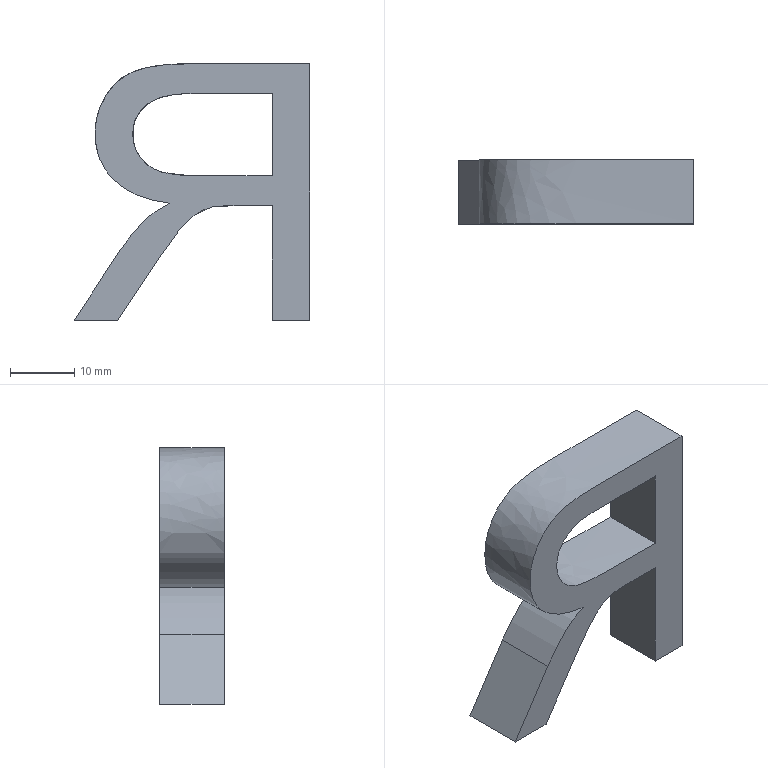Part | NX | features solid 2 | 1 solid | 13 faces | box 36.727 x 10 x 40 mm | volume 6487 mm3 | plane 8 | spline 5
STEP:
#1=CARTESIAN_POINT('',(182.141,850.,-144.665));
#2=VERTEX_POINT('',#1);
#3=CARTESIAN_POINT('',(182.141,850.,-157.484));
#4=VERTEX_POINT('',#3);
#5=CARTESIAN_POINT('',(182.141,850.,-144.665));
#6=CARTESIAN_POINT('',(182.141,850.,-148.938));
#7=CARTESIAN_POINT('',(182.141,850.,-153.211));
#8=CARTESIAN_POINT('',(182.141,850.,-157.484));
#9=B_SPLINE_CURVE_WITH_KNOTS('',3,(#5,#6,#7,#8),.UNSPECIFIED.,.F.,.F.,(4,4),(0.,0.1987),.PIECEWISE_BEZIER_KNOTS.);
#10=EDGE_CURVE('',#2,#4,#9,.T.);
#11=ORIENTED_EDGE('',*,*,#10,.F.);
#12=CARTESIAN_POINT('',(182.141,860.,-144.665));
#13=VERTEX_POINT('',#12);
#14=CARTESIAN_POINT('',(182.141,860.,-144.665));
#15=DIRECTION('',(0.,-1.,0.));
#16=VECTOR('',#15,1000.);
#17=LINE('',#14,#16);
#18=EDGE_CURVE('',#2,#13,#17,.F.);
#19=ORIENTED_EDGE('',*,*,#18,.T.);
#20=CARTESIAN_POINT('',(182.141,860.,-157.484));
#21=VERTEX_POINT('',#20);
#22=CARTESIAN_POINT('',(182.141,860.,-144.665));
#23=CARTESIAN_POINT('',(182.141,860.,-148.938));
#24=CARTESIAN_POINT('',(182.141,860.,-153.211));
#25=CARTESIAN_POINT('',(182.141,860.,-157.484));
#26=B_SPLINE_CURVE_WITH_KNOTS('',3,(#22,#23,#24,#25),.UNSPECIFIED.,.F.,.F.,(4,4),(0.,0.1987),.PIECEWISE_BEZIER_KNOTS.);
#27=EDGE_CURVE('',#13,#21,#26,.T.);
#28=ORIENTED_EDGE('',*,*,#27,.T.);
#29=CARTESIAN_POINT('',(182.141,860.,-157.484));
#30=DIRECTION('',(0.,-1.,0.));
#31=VECTOR('',#30,1000.);
#32=LINE('',#29,#31);
#33=EDGE_CURVE('',#21,#4,#32,.T.);
#34=ORIENTED_EDGE('',*,*,#33,.T.);
#35=EDGE_LOOP('',(#11,#19,#28,#34));
#36=FACE_BOUND('',#35,.T.);
#37=CARTESIAN_POINT('',(182.141,860.,-144.665));
#38=DIRECTION('',(-1.,0.,0.));
#39=DIRECTION('',(0.,-1.,0.));
#40=AXIS2_PLACEMENT_3D('',#37,#38,#39);
#41=PLANE('',#40);
#42=ADVANCED_FACE('',(#36),#41,.T.);
#43=CARTESIAN_POINT('',(182.141,850.,-180.));
#44=VERTEX_POINT('',#43);
#45=CARTESIAN_POINT('',(188.,850.,-180.));
#46=VERTEX_POINT('',#45);
#47=CARTESIAN_POINT('',(182.141,850.,-180.));
#48=CARTESIAN_POINT('',(184.094,850.,-180.));
#49=CARTESIAN_POINT('',(186.047,850.,-180.));
#50=CARTESIAN_POINT('',(188.,850.,-180.));
#51=B_SPLINE_CURVE_WITH_KNOTS('',3,(#47,#48,#49,#50),.UNSPECIFIED.,.F.,.F.,(4,4),(0.,0.02515),.PIECEWISE_BEZIER_KNOTS.);
#52=EDGE_CURVE('',#44,#46,#51,.T.);
#53=ORIENTED_EDGE('',*,*,#52,.F.);
#54=CARTESIAN_POINT('',(182.141,860.,-180.));
#55=VERTEX_POINT('',#54);
#56=CARTESIAN_POINT('',(182.141,860.,-180.));
#57=DIRECTION('',(0.,-1.,0.));
#58=VECTOR('',#57,1000.);
#59=LINE('',#56,#58);
#60=EDGE_CURVE('',#55,#44,#59,.T.);
#61=ORIENTED_EDGE('',*,*,#60,.F.);
#62=CARTESIAN_POINT('',(188.,860.,-180.));
#63=VERTEX_POINT('',#62);
#64=CARTESIAN_POINT('',(182.141,860.,-180.));
#65=CARTESIAN_POINT('',(184.094,860.,-180.));
#66=CARTESIAN_POINT('',(186.047,860.,-180.));
#67=CARTESIAN_POINT('',(188.,860.,-180.));
#68=B_SPLINE_CURVE_WITH_KNOTS('',3,(#64,#65,#66,#67),.UNSPECIFIED.,.F.,.F.,(4,4),(0.,0.02515),.PIECEWISE_BEZIER_KNOTS.);
#69=EDGE_CURVE('',#55,#63,#68,.T.);
#70=ORIENTED_EDGE('',*,*,#69,.T.);
#71=CARTESIAN_POINT('',(188.,860.,-180.));
#72=DIRECTION('',(0.,-1.,0.));
#73=VECTOR('',#72,1000.);
#74=LINE('',#71,#73);
#75=EDGE_CURVE('',#63,#46,#74,.T.);
#76=ORIENTED_EDGE('',*,*,#75,.T.);
#77=EDGE_LOOP('',(#53,#61,#70,#76));
#78=FACE_BOUND('',#77,.T.);
#79=CARTESIAN_POINT('',(182.141,860.,-180.));
#80=DIRECTION('',(0.,0.,-1.));
#81=DIRECTION('',(0.,-1.,0.));
#82=AXIS2_PLACEMENT_3D('',#79,#80,#81);
#83=PLANE('',#82);
#84=ADVANCED_FACE('',(#78),#83,.T.);
#85=CARTESIAN_POINT('',(188.,850.,-140.));
#86=VERTEX_POINT('',#85);
#87=CARTESIAN_POINT('',(188.,850.,-180.));
#88=CARTESIAN_POINT('',(188.,850.,-166.667));
#89=CARTESIAN_POINT('',(188.,850.,-153.333));
#90=CARTESIAN_POINT('',(188.,850.,-140.));
#91=B_SPLINE_CURVE_WITH_KNOTS('',3,(#87,#88,#89,#90),.UNSPECIFIED.,.F.,.F.,(4,4),(0.02515,0.1968),.PIECEWISE_BEZIER_KNOTS.);
#92=EDGE_CURVE('',#46,#86,#91,.T.);
#93=ORIENTED_EDGE('',*,*,#92,.F.);
#94=ORIENTED_EDGE('',*,*,#75,.F.);
#95=CARTESIAN_POINT('',(188.,860.,-140.));
#96=VERTEX_POINT('',#95);
#97=CARTESIAN_POINT('',(188.,860.,-180.));
#98=CARTESIAN_POINT('',(188.,860.,-166.667));
#99=CARTESIAN_POINT('',(188.,860.,-153.333));
#100=CARTESIAN_POINT('',(188.,860.,-140.));
#101=B_SPLINE_CURVE_WITH_KNOTS('',3,(#97,#98,#99,#100),.UNSPECIFIED.,.F.,.F.,(4,4),(0.02515,0.1968),.PIECEWISE_BEZIER_KNOTS.);
#102=EDGE_CURVE('',#63,#96,#101,.T.);
#103=ORIENTED_EDGE('',*,*,#102,.T.);
#104=CARTESIAN_POINT('',(188.,860.,-140.));
#105=DIRECTION('',(0.,-1.,0.));
#106=VECTOR('',#105,1000.);
#107=LINE('',#104,#106);
#108=EDGE_CURVE('',#96,#86,#107,.T.);
#109=ORIENTED_EDGE('',*,*,#108,.T.);
#110=EDGE_LOOP('',(#93,#94,#103,#109));
#111=FACE_BOUND('',#110,.T.);
#112=CARTESIAN_POINT('',(188.,860.,-180.));
#113=DIRECTION('',(1.,0.,0.));
#114=DIRECTION('',(0.,1.,0.));
#115=AXIS2_PLACEMENT_3D('',#112,#113,#114);
#116=PLANE('',#115);
#117=ADVANCED_FACE('',(#111),#116,.T.);
#118=CARTESIAN_POINT('',(166.203,850.,-161.751));
#119=VERTEX_POINT('',#118);
#120=CARTESIAN_POINT('',(188.,850.,-140.));
#121=CARTESIAN_POINT('',(181.759,850.,-140.));
#122=CARTESIAN_POINT('',(175.518,850.,-140.));
#123=CARTESIAN_POINT('',(165.575,850.,-140.));
#124=CARTESIAN_POINT('',(162.776,850.,-140.398));
#125=CARTESIAN_POINT('',(158.92,850.,-141.817));
#126=CARTESIAN_POINT('',(157.407,850.,-143.105));
#127=CARTESIAN_POINT('',(155.106,850.,-146.726));
#128=CARTESIAN_POINT('',(154.532,850.,-148.719));
#129=CARTESIAN_POINT('',(154.532,850.,-153.767));
#130=CARTESIAN_POINT('',(155.48,850.,-156.138));
#131=CARTESIAN_POINT('',(159.297,850.,-160.015));
#132=CARTESIAN_POINT('',(162.226,850.,-161.262));
#133=CARTESIAN_POINT('',(166.203,850.,-161.751));
#134=B_SPLINE_CURVE_WITH_KNOTS('',3,(#120,#121,#122,#123,#124,#125,#126,#127,#128,#129,#130,#131,#132,#133),.UNSPECIFIED.,.F.,.F.,(4,2,2,2,2,2,4),(0.1968,0.2772,0.3249,0.3733,0.4221,0.4858,0.5493),.UNSPECIFIED.);
#135=EDGE_CURVE('',#86,#119,#134,.T.);
#136=ORIENTED_EDGE('',*,*,#135,.F.);
#137=ORIENTED_EDGE('',*,*,#108,.F.);
#138=CARTESIAN_POINT('',(166.203,860.,-161.751));
#139=VERTEX_POINT('',#138);
#140=CARTESIAN_POINT('',(188.,860.,-140.));
#141=CARTESIAN_POINT('',(181.759,860.,-140.));
#142=CARTESIAN_POINT('',(175.518,860.,-140.));
#143=CARTESIAN_POINT('',(165.575,860.,-140.));
#144=CARTESIAN_POINT('',(162.776,860.,-140.398));
#145=CARTESIAN_POINT('',(158.92,860.,-141.817));
#146=CARTESIAN_POINT('',(157.407,860.,-143.105));
#147=CARTESIAN_POINT('',(155.106,860.,-146.726));
#148=CARTESIAN_POINT('',(154.532,860.,-148.719));
#149=CARTESIAN_POINT('',(154.532,860.,-153.767));
#150=CARTESIAN_POINT('',(155.48,860.,-156.138));
#151=CARTESIAN_POINT('',(159.297,860.,-160.015));
#152=CARTESIAN_POINT('',(162.226,860.,-161.262));
#153=CARTESIAN_POINT('',(166.203,860.,-161.751));
#154=B_SPLINE_CURVE_WITH_KNOTS('',3,(#140,#141,#142,#143,#144,#145,#146,#147,#148,#149,#150,#151,#152,#153),.UNSPECIFIED.,.F.,.F.,(4,2,2,2,2,2,4),(0.1968,0.2772,0.3249,0.3733,0.4221,0.4858,0.5493),.UNSPECIFIED.);
#155=EDGE_CURVE('',#96,#139,#154,.T.);
#156=ORIENTED_EDGE('',*,*,#155,.T.);
#157=CARTESIAN_POINT('',(166.203,860.,-161.751));
#158=DIRECTION('',(0.,-1.,0.));
#159=VECTOR('',#158,1000.);
#160=LINE('',#157,#159);
#161=EDGE_CURVE('',#139,#119,#160,.T.);
#162=ORIENTED_EDGE('',*,*,#161,.T.);
#163=EDGE_LOOP('',(#136,#137,#156,#162));
#164=FACE_BOUND('',#163,.T.);
#165=CARTESIAN_POINT('',(188.,860.,-140.));
#166=CARTESIAN_POINT('',(188.,850.,-140.));
#167=CARTESIAN_POINT('',(186.289,860.,-140.));
#168=CARTESIAN_POINT('',(186.289,850.,-140.));
#169=CARTESIAN_POINT('',(182.869,860.,-140.001));
#170=CARTESIAN_POINT('',(182.869,850.,-140.001));
#171=CARTESIAN_POINT('',(177.726,860.,-139.996));
#172=CARTESIAN_POINT('',(177.726,850.,-139.996));
#173=CARTESIAN_POINT('',(172.631,860.,-140.014));
#174=CARTESIAN_POINT('',(172.631,850.,-140.014));
#175=CARTESIAN_POINT('',(167.357,860.,-139.948));
#176=CARTESIAN_POINT('',(167.357,850.,-139.948));
#177=CARTESIAN_POINT('',(163.179,860.,-140.38));
#178=CARTESIAN_POINT('',(163.179,850.,-140.38));
#179=CARTESIAN_POINT('',(160.262,860.,-141.195));
#180=CARTESIAN_POINT('',(160.262,850.,-141.195));
#181=CARTESIAN_POINT('',(158.009,860.,-142.63));
#182=CARTESIAN_POINT('',(158.009,850.,-142.63));
#183=CARTESIAN_POINT('',(156.179,860.,-144.813));
#184=CARTESIAN_POINT('',(156.179,850.,-144.813));
#185=CARTESIAN_POINT('',(154.936,860.,-147.421));
#186=CARTESIAN_POINT('',(154.936,850.,-147.421));
#187=CARTESIAN_POINT('',(154.434,860.,-150.223));
#188=CARTESIAN_POINT('',(154.434,850.,-150.223));
#189=CARTESIAN_POINT('',(154.623,860.,-153.18));
#190=CARTESIAN_POINT('',(154.623,850.,-153.18));
#191=CARTESIAN_POINT('',(155.493,860.,-155.681));
#192=CARTESIAN_POINT('',(155.493,850.,-155.681));
#193=CARTESIAN_POINT('',(157.046,860.,-157.904));
#194=CARTESIAN_POINT('',(157.046,850.,-157.904));
#195=CARTESIAN_POINT('',(160.058,860.,-160.367));
#196=CARTESIAN_POINT('',(160.058,850.,-160.367));
#197=CARTESIAN_POINT('',(163.443,860.,-161.412));
#198=CARTESIAN_POINT('',(163.443,850.,-161.412));
#199=CARTESIAN_POINT('',(166.203,860.,-161.751));
#200=CARTESIAN_POINT('',(166.203,850.,-161.751));
#201=B_SPLINE_SURFACE_WITH_KNOTS('',3,1,((#165,#166),(#167,#168),(#169,#170),(#171,#172),(#173,#174),(#175,#176),(#177,#178),(#179,#180),(#181,#182),(#183,#184),(#185,#186),(#187,#188),(#189,#190),(#191,#192),(#193,#194),(#195,#196),(#197,#198),(#199,#200)),.SURF_OF_LINEAR_EXTRUSION.,.F.,.F.,.F.,(4,1,1,1,1,1,1,1,1,1,1,1,1,1,1,4),(2,2),(0.1968,0.2189,0.2409,0.2629,0.285,0.307,0.329,0.351,0.3731,0.3951,0.4171,0.4392,0.4612,0.4832,0.5053,0.5493),(0.,1.),.UNSPECIFIED.);
#202=ADVANCED_FACE('',(#164),#201,.T.);
#203=CARTESIAN_POINT('',(158.402,850.,-169.109));
#204=VERTEX_POINT('',#203);
#205=CARTESIAN_POINT('',(166.203,850.,-161.751));
#206=CARTESIAN_POINT('',(164.765,850.,-162.455));
#207=CARTESIAN_POINT('',(163.663,850.,-163.128));
#208=CARTESIAN_POINT('',(162.939,850.,-163.781));
#209=CARTESIAN_POINT('',(161.338,850.,-165.224));
#210=CARTESIAN_POINT('',(159.824,850.,-167.013));
#211=CARTESIAN_POINT('',(158.402,850.,-169.109));
#212=B_SPLINE_CURVE_WITH_KNOTS('',3,(#205,#206,#207,#208,#209,#210,#211),.UNSPECIFIED.,.F.,.F.,(4,3,4),(0.5493,0.5699,0.6072),.PIECEWISE_BEZIER_KNOTS.);
#213=EDGE_CURVE('',#119,#204,#212,.T.);
#214=ORIENTED_EDGE('',*,*,#213,.F.);
#215=ORIENTED_EDGE('',*,*,#161,.F.);
#216=CARTESIAN_POINT('',(158.402,860.,-169.109));
#217=VERTEX_POINT('',#216);
#218=CARTESIAN_POINT('',(166.203,860.,-161.751));
#219=CARTESIAN_POINT('',(164.765,860.,-162.455));
#220=CARTESIAN_POINT('',(163.663,860.,-163.128));
#221=CARTESIAN_POINT('',(162.939,860.,-163.781));
#222=CARTESIAN_POINT('',(161.338,860.,-165.224));
#223=CARTESIAN_POINT('',(159.824,860.,-167.013));
#224=CARTESIAN_POINT('',(158.402,860.,-169.109));
#225=B_SPLINE_CURVE_WITH_KNOTS('',3,(#218,#219,#220,#221,#222,#223,#224),.UNSPECIFIED.,.F.,.F.,(4,3,4),(0.5493,0.5699,0.6072),.PIECEWISE_BEZIER_KNOTS.);
#226=EDGE_CURVE('',#139,#217,#225,.T.);
#227=ORIENTED_EDGE('',*,*,#226,.T.);
#228=CARTESIAN_POINT('',(158.402,860.,-169.109));
#229=DIRECTION('',(0.,-1.,0.));
#230=VECTOR('',#229,1000.);
#231=LINE('',#228,#230);
#232=EDGE_CURVE('',#217,#204,#231,.T.);
#233=ORIENTED_EDGE('',*,*,#232,.T.);
#234=EDGE_LOOP('',(#214,#215,#227,#233));
#235=FACE_BOUND('',#234,.T.);
#236=CARTESIAN_POINT('',(166.203,860.,-161.751));
#237=CARTESIAN_POINT('',(166.203,850.,-161.751));
#238=CARTESIAN_POINT('',(165.189,860.,-162.247));
#239=CARTESIAN_POINT('',(165.189,850.,-162.247));
#240=CARTESIAN_POINT('',(163.896,860.,-162.98));
#241=CARTESIAN_POINT('',(163.896,850.,-162.98));
#242=CARTESIAN_POINT('',(162.81,860.,-163.876));
#243=CARTESIAN_POINT('',(162.81,850.,-163.876));
#244=CARTESIAN_POINT('',(161.547,860.,-165.109));
#245=CARTESIAN_POINT('',(161.547,850.,-165.109));
#246=CARTESIAN_POINT('',(160.088,860.,-166.759));
#247=CARTESIAN_POINT('',(160.088,850.,-166.759));
#248=CARTESIAN_POINT('',(158.953,860.,-168.297));
#249=CARTESIAN_POINT('',(158.953,850.,-168.297));
#250=CARTESIAN_POINT('',(158.402,860.,-169.109));
#251=CARTESIAN_POINT('',(158.402,850.,-169.109));
#252=B_SPLINE_SURFACE_WITH_KNOTS('',3,1,((#236,#237),(#238,#239),(#240,#241),(#242,#243),(#244,#245),(#246,#247),(#248,#249),(#250,#251)),.SURF_OF_LINEAR_EXTRUSION.,.F.,.F.,.F.,(4,1,1,1,1,4),(2,2),(0.5493,0.5638,0.571,0.5783,0.5927,0.6072),(0.,1.),.UNSPECIFIED.);
#253=ADVANCED_FACE('',(#235),#252,.T.);
#254=CARTESIAN_POINT('',(151.273,850.,-180.));
#255=VERTEX_POINT('',#254);
#256=CARTESIAN_POINT('',(158.402,850.,-169.109));
#257=CARTESIAN_POINT('',(156.025,850.,-172.739));
#258=CARTESIAN_POINT('',(153.649,850.,-176.37));
#259=CARTESIAN_POINT('',(151.273,850.,-180.));
#260=B_SPLINE_CURVE_WITH_KNOTS('',3,(#256,#257,#258,#259),.UNSPECIFIED.,.F.,.F.,(4,4),(0.6072,0.6765),.PIECEWISE_BEZIER_KNOTS.);
#261=EDGE_CURVE('',#204,#255,#260,.T.);
#262=ORIENTED_EDGE('',*,*,#261,.F.);
#263=ORIENTED_EDGE('',*,*,#232,.F.);
#264=CARTESIAN_POINT('',(151.273,860.,-180.));
#265=VERTEX_POINT('',#264);
#266=CARTESIAN_POINT('',(158.402,860.,-169.109));
#267=CARTESIAN_POINT('',(156.025,860.,-172.739));
#268=CARTESIAN_POINT('',(153.649,860.,-176.37));
#269=CARTESIAN_POINT('',(151.273,860.,-180.));
#270=B_SPLINE_CURVE_WITH_KNOTS('',3,(#266,#267,#268,#269),.UNSPECIFIED.,.F.,.F.,(4,4),(0.6072,0.6765),.PIECEWISE_BEZIER_KNOTS.);
#271=EDGE_CURVE('',#217,#265,#270,.T.);
#272=ORIENTED_EDGE('',*,*,#271,.T.);
#273=CARTESIAN_POINT('',(151.273,860.,-180.));
#274=DIRECTION('',(0.,-1.,0.));
#275=VECTOR('',#274,1000.);
#276=LINE('',#273,#275);
#277=EDGE_CURVE('',#265,#255,#276,.T.);
#278=ORIENTED_EDGE('',*,*,#277,.T.);
#279=EDGE_LOOP('',(#262,#263,#272,#278));
#280=FACE_BOUND('',#279,.T.);
#281=CARTESIAN_POINT('',(158.402,860.,-169.109));
#282=DIRECTION('',(-0.8367,0.,0.5476));
#283=DIRECTION('',(0.5476,0.,0.8367));
#284=AXIS2_PLACEMENT_3D('',#281,#282,#283);
#285=PLANE('',#284);
#286=ADVANCED_FACE('',(#280),#285,.T.);
#287=CARTESIAN_POINT('',(158.034,850.,-180.));
#288=VERTEX_POINT('',#287);
#289=CARTESIAN_POINT('',(151.273,850.,-180.));
#290=CARTESIAN_POINT('',(153.527,850.,-180.));
#291=CARTESIAN_POINT('',(155.781,850.,-180.));
#292=CARTESIAN_POINT('',(158.034,850.,-180.));
#293=B_SPLINE_CURVE_WITH_KNOTS('',3,(#289,#290,#291,#292),.UNSPECIFIED.,.F.,.F.,(4,4),(0.6765,0.7125),.PIECEWISE_BEZIER_KNOTS.);
#294=EDGE_CURVE('',#255,#288,#293,.T.);
#295=ORIENTED_EDGE('',*,*,#294,.F.);
#296=ORIENTED_EDGE('',*,*,#277,.F.);
#297=CARTESIAN_POINT('',(158.034,860.,-180.));
#298=VERTEX_POINT('',#297);
#299=CARTESIAN_POINT('',(151.273,860.,-180.));
#300=CARTESIAN_POINT('',(153.527,860.,-180.));
#301=CARTESIAN_POINT('',(155.781,860.,-180.));
#302=CARTESIAN_POINT('',(158.034,860.,-180.));
#303=B_SPLINE_CURVE_WITH_KNOTS('',3,(#299,#300,#301,#302),.UNSPECIFIED.,.F.,.F.,(4,4),(0.6765,0.7125),.PIECEWISE_BEZIER_KNOTS.);
#304=EDGE_CURVE('',#265,#298,#303,.T.);
#305=ORIENTED_EDGE('',*,*,#304,.T.);
#306=CARTESIAN_POINT('',(158.034,860.,-180.));
#307=DIRECTION('',(0.,-1.,0.));
#308=VECTOR('',#307,1000.);
#309=LINE('',#306,#308);
#310=EDGE_CURVE('',#298,#288,#309,.T.);
#311=ORIENTED_EDGE('',*,*,#310,.T.);
#312=EDGE_LOOP('',(#295,#296,#305,#311));
#313=FACE_BOUND('',#312,.T.);
#314=CARTESIAN_POINT('',(151.273,860.,-180.));
#315=DIRECTION('',(0.,0.,-1.));
#316=DIRECTION('',(0.,-1.,0.));
#317=AXIS2_PLACEMENT_3D('',#314,#315,#316);
#318=PLANE('',#317);
#319=ADVANCED_FACE('',(#313),#318,.T.);
#320=CARTESIAN_POINT('',(172.765,850.,-162.333));
#321=VERTEX_POINT('',#320);
#322=CARTESIAN_POINT('',(158.034,850.,-180.));
#323=CARTESIAN_POINT('',(159.865,850.,-177.226));
#324=CARTESIAN_POINT('',(161.695,850.,-174.453));
#325=CARTESIAN_POINT('',(163.541,850.,-171.689));
#326=CARTESIAN_POINT('',(165.132,850.,-169.308));
#327=CARTESIAN_POINT('',(166.432,850.,-167.457));
#328=CARTESIAN_POINT('',(168.499,850.,-164.904));
#329=CARTESIAN_POINT('',(169.415,850.,-163.985));
#330=CARTESIAN_POINT('',(170.246,850.,-163.457));
#331=CARTESIAN_POINT('',(171.052,850.,-162.945));
#332=CARTESIAN_POINT('',(171.893,850.,-162.577));
#333=CARTESIAN_POINT('',(172.765,850.,-162.333));
#334=B_SPLINE_CURVE_WITH_KNOTS('',3,(#322,#323,#324,#325,#326,#327,#328,#329,#330,#331,#332,#333),.UNSPECIFIED.,.F.,.F.,(4,3,2,3,4),(0.7125,0.7656,0.8017,0.8373,0.8523),.UNSPECIFIED.);
#335=EDGE_CURVE('',#288,#321,#334,.T.);
#336=ORIENTED_EDGE('',*,*,#335,.F.);
#337=ORIENTED_EDGE('',*,*,#310,.F.);
#338=CARTESIAN_POINT('',(172.765,860.,-162.333));
#339=VERTEX_POINT('',#338);
#340=CARTESIAN_POINT('',(158.034,860.,-180.));
#341=CARTESIAN_POINT('',(159.865,860.,-177.226));
#342=CARTESIAN_POINT('',(161.695,860.,-174.453));
#343=CARTESIAN_POINT('',(163.541,860.,-171.689));
#344=CARTESIAN_POINT('',(165.132,860.,-169.308));
#345=CARTESIAN_POINT('',(166.432,860.,-167.457));
#346=CARTESIAN_POINT('',(168.499,860.,-164.904));
#347=CARTESIAN_POINT('',(169.415,860.,-163.985));
#348=CARTESIAN_POINT('',(170.246,860.,-163.457));
#349=CARTESIAN_POINT('',(171.052,860.,-162.945));
#350=CARTESIAN_POINT('',(171.893,860.,-162.577));
#351=CARTESIAN_POINT('',(172.765,860.,-162.333));
#352=B_SPLINE_CURVE_WITH_KNOTS('',3,(#340,#341,#342,#343,#344,#345,#346,#347,#348,#349,#350,#351),.UNSPECIFIED.,.F.,.F.,(4,3,2,3,4),(0.7125,0.7656,0.8017,0.8373,0.8523),.UNSPECIFIED.);
#353=EDGE_CURVE('',#298,#339,#352,.T.);
#354=ORIENTED_EDGE('',*,*,#353,.T.);
#355=CARTESIAN_POINT('',(172.765,860.,-162.333));
#356=DIRECTION('',(0.,-1.,0.));
#357=VECTOR('',#356,1000.);
#358=LINE('',#355,#357);
#359=EDGE_CURVE('',#339,#321,#358,.T.);
#360=ORIENTED_EDGE('',*,*,#359,.T.);
#361=EDGE_LOOP('',(#336,#337,#354,#360));
#362=FACE_BOUND('',#361,.T.);
#363=CARTESIAN_POINT('',(158.034,860.,-180.));
#364=CARTESIAN_POINT('',(158.034,850.,-180.));
#365=CARTESIAN_POINT('',(158.637,860.,-179.087));
#366=CARTESIAN_POINT('',(158.637,850.,-179.087));
#367=CARTESIAN_POINT('',(159.841,860.,-177.262));
#368=CARTESIAN_POINT('',(159.841,850.,-177.262));
#369=CARTESIAN_POINT('',(161.354,860.,-174.976));
#370=CARTESIAN_POINT('',(161.354,850.,-174.976));
#371=CARTESIAN_POINT('',(162.406,860.,-173.392));
#372=CARTESIAN_POINT('',(162.406,850.,-173.392));
#373=CARTESIAN_POINT('',(163.024,860.,-172.465));
#374=CARTESIAN_POINT('',(163.024,850.,-172.465));
#375=CARTESIAN_POINT('',(163.445,860.,-171.833));
#376=CARTESIAN_POINT('',(163.445,850.,-171.833));
#377=CARTESIAN_POINT('',(164.03,860.,-170.959));
#378=CARTESIAN_POINT('',(164.03,850.,-170.959));
#379=CARTESIAN_POINT('',(164.749,860.,-169.899));
#380=CARTESIAN_POINT('',(164.749,850.,-169.899));
#381=CARTESIAN_POINT('',(165.934,860.,-168.188));
#382=CARTESIAN_POINT('',(165.934,850.,-168.188));
#383=CARTESIAN_POINT('',(167.083,860.,-166.632));
#384=CARTESIAN_POINT('',(167.083,850.,-166.632));
#385=CARTESIAN_POINT('',(168.065,860.,-165.451));
#386=CARTESIAN_POINT('',(168.065,850.,-165.451));
#387=CARTESIAN_POINT('',(168.771,860.,-164.682));
#388=CARTESIAN_POINT('',(168.771,850.,-164.682));
#389=CARTESIAN_POINT('',(169.335,860.,-164.15));
#390=CARTESIAN_POINT('',(169.335,850.,-164.15));
#391=CARTESIAN_POINT('',(169.75,860.,-163.803));
#392=CARTESIAN_POINT('',(169.75,850.,-163.803));
#393=CARTESIAN_POINT('',(170.048,860.,-163.588));
#394=CARTESIAN_POINT('',(170.048,850.,-163.588));
#395=CARTESIAN_POINT('',(170.18,860.,-163.497));
#396=CARTESIAN_POINT('',(170.18,850.,-163.497));
#397=CARTESIAN_POINT('',(170.683,860.,-163.185));
#398=CARTESIAN_POINT('',(170.683,850.,-163.185));
#399=CARTESIAN_POINT('',(171.503,860.,-162.757));
#400=CARTESIAN_POINT('',(171.503,850.,-162.757));
#401=CARTESIAN_POINT('',(172.257,860.,-162.475));
#402=CARTESIAN_POINT('',(172.257,850.,-162.475));
#403=CARTESIAN_POINT('',(172.765,860.,-162.333));
#404=CARTESIAN_POINT('',(172.765,850.,-162.333));
#405=B_SPLINE_SURFACE_WITH_KNOTS('',3,1,((#363,#364),(#365,#366),(#367,#368),(#369,#370),(#371,#372),(#373,#374),(#375,#376),(#377,#378),(#379,#380),(#381,#382),(#383,#384),(#385,#386),(#387,#388),(#389,#390),(#391,#392),(#393,#394),(#395,#396),(#397,#398),(#399,#400),(#401,#402),(#403,#404)),.SURF_OF_LINEAR_EXTRUSION.,.F.,.F.,.F.,(4,1,1,1,1,1,1,1,1,1,1,1,1,1,1,1,1,1,4),(2,2),(0.7125,0.73,0.7475,0.7562,0.7606,0.7649,0.7693,0.7737,0.7824,0.7999,0.8086,0.8173,0.8261,0.8305,0.8348,0.837,0.8392,0.8436,0.8523),(0.,1.),.UNSPECIFIED.);
#406=ADVANCED_FACE('',(#362),#405,.T.);
#407=CARTESIAN_POINT('',(182.141,850.,-162.134));
#408=VERTEX_POINT('',#407);
#409=CARTESIAN_POINT('',(172.765,850.,-162.333));
#410=CARTESIAN_POINT('',(173.361,850.,-162.241));
#411=CARTESIAN_POINT('',(174.371,850.,-162.164));
#412=CARTESIAN_POINT('',(175.794,850.,-162.152));
#413=CARTESIAN_POINT('',(177.909,850.,-162.134));
#414=CARTESIAN_POINT('',(180.025,850.,-162.134));
#415=CARTESIAN_POINT('',(182.141,850.,-162.134));
#416=B_SPLINE_CURVE_WITH_KNOTS('',3,(#409,#410,#411,#412,#413,#414,#415),.UNSPECIFIED.,.F.,.F.,(4,3,4),(0.8523,0.8688,0.9032),.PIECEWISE_BEZIER_KNOTS.);
#417=EDGE_CURVE('',#321,#408,#416,.T.);
#418=ORIENTED_EDGE('',*,*,#417,.F.);
#419=ORIENTED_EDGE('',*,*,#359,.F.);
#420=CARTESIAN_POINT('',(182.141,860.,-162.134));
#421=VERTEX_POINT('',#420);
#422=CARTESIAN_POINT('',(172.765,860.,-162.333));
#423=CARTESIAN_POINT('',(173.361,860.,-162.241));
#424=CARTESIAN_POINT('',(174.371,860.,-162.164));
#425=CARTESIAN_POINT('',(175.794,860.,-162.152));
#426=CARTESIAN_POINT('',(177.909,860.,-162.134));
#427=CARTESIAN_POINT('',(180.025,860.,-162.134));
#428=CARTESIAN_POINT('',(182.141,860.,-162.134));
#429=B_SPLINE_CURVE_WITH_KNOTS('',3,(#422,#423,#424,#425,#426,#427,#428),.UNSPECIFIED.,.F.,.F.,(4,3,4),(0.8523,0.8688,0.9032),.PIECEWISE_BEZIER_KNOTS.);
#430=EDGE_CURVE('',#339,#421,#429,.T.);
#431=ORIENTED_EDGE('',*,*,#430,.T.);
#432=CARTESIAN_POINT('',(182.141,860.,-162.134));
#433=DIRECTION('',(0.,-1.,0.));
#434=VECTOR('',#433,1000.);
#435=LINE('',#432,#434);
#436=EDGE_CURVE('',#421,#408,#435,.T.);
#437=ORIENTED_EDGE('',*,*,#436,.T.);
#438=EDGE_LOOP('',(#418,#419,#431,#437));
#439=FACE_BOUND('',#438,.T.);
#440=CARTESIAN_POINT('',(172.765,860.,-162.333));
#441=CARTESIAN_POINT('',(172.765,850.,-162.333));
#442=CARTESIAN_POINT('',(172.995,860.,-162.297));
#443=CARTESIAN_POINT('',(172.995,850.,-162.297));
#444=CARTESIAN_POINT('',(173.591,860.,-162.231));
#445=CARTESIAN_POINT('',(173.591,850.,-162.231));
#446=CARTESIAN_POINT('',(174.586,860.,-162.173));
#447=CARTESIAN_POINT('',(174.586,850.,-162.173));
#448=CARTESIAN_POINT('',(175.689,860.,-162.151));
#449=CARTESIAN_POINT('',(175.689,850.,-162.151));
#450=CARTESIAN_POINT('',(176.472,860.,-162.147));
#451=CARTESIAN_POINT('',(176.472,850.,-162.147));
#452=CARTESIAN_POINT('',(177.84,860.,-162.138));
#453=CARTESIAN_POINT('',(177.84,850.,-162.138));
#454=CARTESIAN_POINT('',(179.795,860.,-162.134));
#455=CARTESIAN_POINT('',(179.795,850.,-162.134));
#456=CARTESIAN_POINT('',(181.359,860.,-162.134));
#457=CARTESIAN_POINT('',(181.359,850.,-162.134));
#458=CARTESIAN_POINT('',(182.141,860.,-162.134));
#459=CARTESIAN_POINT('',(182.141,850.,-162.134));
#460=B_SPLINE_SURFACE_WITH_KNOTS('',3,1,((#440,#441),(#442,#443),(#444,#445),(#446,#447),(#448,#449),(#450,#451),(#452,#453),(#454,#455),(#456,#457),(#458,#459)),.SURF_OF_LINEAR_EXTRUSION.,.F.,.F.,.F.,(4,1,1,1,1,1,1,4),(2,2),(0.8523,0.8587,0.865,0.8682,0.8714,0.8777,0.8904,0.9032),(0.,1.),.UNSPECIFIED.);
#461=ADVANCED_FACE('',(#439),#460,.T.);
#462=CARTESIAN_POINT('',(182.141,850.,-162.134));
#463=CARTESIAN_POINT('',(182.141,850.,-168.089));
#464=CARTESIAN_POINT('',(182.141,850.,-174.045));
#465=CARTESIAN_POINT('',(182.141,850.,-180.));
#466=B_SPLINE_CURVE_WITH_KNOTS('',3,(#462,#463,#464,#465),.UNSPECIFIED.,.F.,.F.,(4,4),(0.9032,1.),.PIECEWISE_BEZIER_KNOTS.);
#467=EDGE_CURVE('',#408,#44,#466,.T.);
#468=ORIENTED_EDGE('',*,*,#467,.F.);
#469=ORIENTED_EDGE('',*,*,#436,.F.);
#470=CARTESIAN_POINT('',(182.141,860.,-162.134));
#471=CARTESIAN_POINT('',(182.141,860.,-168.089));
#472=CARTESIAN_POINT('',(182.141,860.,-174.045));
#473=CARTESIAN_POINT('',(182.141,860.,-180.));
#474=B_SPLINE_CURVE_WITH_KNOTS('',3,(#470,#471,#472,#473),.UNSPECIFIED.,.F.,.F.,(4,4),(0.9032,1.),.PIECEWISE_BEZIER_KNOTS.);
#475=EDGE_CURVE('',#421,#55,#474,.T.);
#476=ORIENTED_EDGE('',*,*,#475,.T.);
#477=ORIENTED_EDGE('',*,*,#60,.T.);
#478=EDGE_LOOP('',(#468,#469,#476,#477));
#479=FACE_BOUND('',#478,.T.);
#480=CARTESIAN_POINT('',(182.141,860.,-162.134));
#481=DIRECTION('',(-1.,0.,0.));
#482=DIRECTION('',(0.,-1.,0.));
#483=AXIS2_PLACEMENT_3D('',#480,#481,#482);
#484=PLANE('',#483);
#485=ADVANCED_FACE('',(#479),#484,.T.);
#486=CARTESIAN_POINT('',(182.141,850.,-157.484));
#487=CARTESIAN_POINT('',(178.221,850.,-157.484));
#488=CARTESIAN_POINT('',(174.3,850.,-157.484));
#489=CARTESIAN_POINT('',(167.87,850.,-157.484));
#490=CARTESIAN_POINT('',(165.927,850.,-157.254));
#491=CARTESIAN_POINT('',(163.217,850.,-156.299));
#492=CARTESIAN_POINT('',(162.164,850.,-155.511));
#493=CARTESIAN_POINT('',(161.443,850.,-154.452));
#494=CARTESIAN_POINT('',(160.727,850.,-153.4));
#495=CARTESIAN_POINT('',(160.39,850.,-152.237));
#496=CARTESIAN_POINT('',(160.39,850.,-149.147));
#497=CARTESIAN_POINT('',(161.078,850.,-147.648));
#498=CARTESIAN_POINT('',(163.86,850.,-145.29));
#499=CARTESIAN_POINT('',(166.065,850.,-144.681));
#500=CARTESIAN_POINT('',(173.412,850.,-144.643));
#501=CARTESIAN_POINT('',(177.777,850.,-144.665));
#502=CARTESIAN_POINT('',(182.141,850.,-144.665));
#503=B_SPLINE_CURVE_WITH_KNOTS('',3,(#486,#487,#488,#489,#490,#491,#492,#493,#494,#495,#496,#497,#498,#499,#500,#501,#502),.UNSPECIFIED.,.F.,.F.,(4,2,2,3,2,2,2,4),(0.1987,0.3811,0.4978,0.616,0.6824,0.7757,0.8667,1.),.UNSPECIFIED.);
#504=EDGE_CURVE('',#4,#2,#503,.T.);
#505=ORIENTED_EDGE('',*,*,#504,.F.);
#506=ORIENTED_EDGE('',*,*,#33,.F.);
#507=CARTESIAN_POINT('',(182.141,860.,-157.484));
#508=CARTESIAN_POINT('',(178.221,860.,-157.484));
#509=CARTESIAN_POINT('',(174.3,860.,-157.484));
#510=CARTESIAN_POINT('',(167.87,860.,-157.484));
#511=CARTESIAN_POINT('',(165.927,860.,-157.254));
#512=CARTESIAN_POINT('',(163.217,860.,-156.299));
#513=CARTESIAN_POINT('',(162.164,860.,-155.511));
#514=CARTESIAN_POINT('',(161.443,860.,-154.452));
#515=CARTESIAN_POINT('',(160.727,860.,-153.4));
#516=CARTESIAN_POINT('',(160.39,860.,-152.237));
#517=CARTESIAN_POINT('',(160.39,860.,-149.147));
#518=CARTESIAN_POINT('',(161.078,860.,-147.648));
#519=CARTESIAN_POINT('',(163.86,860.,-145.29));
#520=CARTESIAN_POINT('',(166.065,860.,-144.681));
#521=CARTESIAN_POINT('',(173.412,860.,-144.643));
#522=CARTESIAN_POINT('',(177.777,860.,-144.665));
#523=CARTESIAN_POINT('',(182.141,860.,-144.665));
#524=B_SPLINE_CURVE_WITH_KNOTS('',3,(#507,#508,#509,#510,#511,#512,#513,#514,#515,#516,#517,#518,#519,#520,#521,#522,#523),.UNSPECIFIED.,.F.,.F.,(4,2,2,3,2,2,2,4),(0.1987,0.3811,0.4978,0.616,0.6824,0.7757,0.8667,1.),.UNSPECIFIED.);
#525=EDGE_CURVE('',#21,#13,#524,.T.);
#526=ORIENTED_EDGE('',*,*,#525,.T.);
#527=ORIENTED_EDGE('',*,*,#18,.F.);
#528=EDGE_LOOP('',(#505,#506,#526,#527));
#529=FACE_BOUND('',#528,.T.);
#530=CARTESIAN_POINT('',(182.141,860.,-157.484));
#531=CARTESIAN_POINT('',(182.141,850.,-157.484));
#532=CARTESIAN_POINT('',(179.988,860.,-157.484));
#533=CARTESIAN_POINT('',(179.988,850.,-157.484));
#534=CARTESIAN_POINT('',(176.748,860.,-157.488));
#535=CARTESIAN_POINT('',(176.748,850.,-157.488));
#536=CARTESIAN_POINT('',(172.466,860.,-157.477));
#537=CARTESIAN_POINT('',(172.466,850.,-157.477));
#538=CARTESIAN_POINT('',(169.16,860.,-157.51));
#539=CARTESIAN_POINT('',(169.16,850.,-157.51));
#540=CARTESIAN_POINT('',(166.457,860.,-157.289));
#541=CARTESIAN_POINT('',(166.457,850.,-157.289));
#542=CARTESIAN_POINT('',(164.451,860.,-156.813));
#543=CARTESIAN_POINT('',(164.451,850.,-156.813));
#544=CARTESIAN_POINT('',(163.181,860.,-156.162));
#545=CARTESIAN_POINT('',(163.181,850.,-156.162));
#546=CARTESIAN_POINT('',(162.316,860.,-155.485));
#547=CARTESIAN_POINT('',(162.316,850.,-155.485));
#548=CARTESIAN_POINT('',(161.84,860.,-154.984));
#549=CARTESIAN_POINT('',(161.84,850.,-154.984));
#550=CARTESIAN_POINT('',(161.567,860.,-154.631));
#551=CARTESIAN_POINT('',(161.567,850.,-154.631));
#552=CARTESIAN_POINT('',(161.387,860.,-154.374));
#553=CARTESIAN_POINT('',(161.387,850.,-154.374));
#554=CARTESIAN_POINT('',(161.116,860.,-153.936));
#555=CARTESIAN_POINT('',(161.116,850.,-153.936));
#556=CARTESIAN_POINT('',(160.868,860.,-153.433));
#557=CARTESIAN_POINT('',(160.868,850.,-153.433));
#558=CARTESIAN_POINT('',(160.552,860.,-152.564));
#559=CARTESIAN_POINT('',(160.552,850.,-152.564));
#560=CARTESIAN_POINT('',(160.357,860.,-151.423));
#561=CARTESIAN_POINT('',(160.357,850.,-151.423));
#562=CARTESIAN_POINT('',(160.427,860.,-149.476));
#563=CARTESIAN_POINT('',(160.427,850.,-149.476));
#564=CARTESIAN_POINT('',(161.27,860.,-147.452));
#565=CARTESIAN_POINT('',(161.27,850.,-147.452));
#566=CARTESIAN_POINT('',(163.501,860.,-145.477));
#567=CARTESIAN_POINT('',(163.501,850.,-145.477));
#568=CARTESIAN_POINT('',(166.582,860.,-144.697));
#569=CARTESIAN_POINT('',(166.582,850.,-144.697));
#570=CARTESIAN_POINT('',(169.836,860.,-144.657));
#571=CARTESIAN_POINT('',(169.836,850.,-144.657));
#572=CARTESIAN_POINT('',(173.123,860.,-144.655));
#573=CARTESIAN_POINT('',(173.123,850.,-144.655));
#574=CARTESIAN_POINT('',(177.22,860.,-144.658));
#575=CARTESIAN_POINT('',(177.22,850.,-144.658));
#576=CARTESIAN_POINT('',(180.501,860.,-144.665));
#577=CARTESIAN_POINT('',(180.501,850.,-144.665));
#578=CARTESIAN_POINT('',(182.141,860.,-144.665));
#579=CARTESIAN_POINT('',(182.141,850.,-144.665));
#580=B_SPLINE_SURFACE_WITH_KNOTS('',3,1,((#530,#531),(#532,#533),(#534,#535),(#536,#537),(#538,#539),(#540,#541),(#542,#543),(#544,#545),(#546,#547),(#548,#549),(#550,#551),(#552,#553),(#554,#555),(#556,#557),(#558,#559),(#560,#561),(#562,#563),(#564,#565),(#566,#567),(#568,#569),(#570,#571),(#572,#573),(#574,#575),(#576,#577),(#578,#579)),.SURF_OF_LINEAR_EXTRUSION.,.F.,.F.,.F.,(4,1,1,1,1,1,1,1,1,1,1,1,1,1,1,1,1,1,1,1,1,1,4),(2,2),(0.1987,0.2989,0.349,0.399,0.4491,0.4992,0.5493,0.5743,0.5994,0.6119,0.6181,0.6244,0.6369,0.6494,0.6745,0.6995,0.7496,0.7997,0.8498,0.8748,0.8998,0.9499,1.),(0.,1.),.UNSPECIFIED.);
#581=ADVANCED_FACE('',(#529),#580,.T.);
#582=ORIENTED_EDGE('',*,*,#69,.F.);
#583=ORIENTED_EDGE('',*,*,#475,.F.);
#584=ORIENTED_EDGE('',*,*,#430,.F.);
#585=ORIENTED_EDGE('',*,*,#353,.F.);
#586=ORIENTED_EDGE('',*,*,#304,.F.);
#587=ORIENTED_EDGE('',*,*,#271,.F.);
#588=ORIENTED_EDGE('',*,*,#226,.F.);
#589=ORIENTED_EDGE('',*,*,#155,.F.);
#590=ORIENTED_EDGE('',*,*,#102,.F.);
#591=EDGE_LOOP('',(#582,#583,#584,#585,#586,#587,#588,#589,#590));
#592=FACE_BOUND('',#591,.T.);
#593=ORIENTED_EDGE('',*,*,#27,.F.);
#594=ORIENTED_EDGE('',*,*,#525,.F.);
#595=EDGE_LOOP('',(#593,#594));
#596=FACE_BOUND('',#595,.T.);
#597=CARTESIAN_POINT('',(156.277,860.,-144.884));
#598=DIRECTION('',(0.,1.,0.));
#599=DIRECTION('',(-1.,0.,0.));
#600=AXIS2_PLACEMENT_3D('',#597,#598,#599);
#601=PLANE('',#600);
#602=ADVANCED_FACE('',(#592,#596),#601,.T.);
#603=ORIENTED_EDGE('',*,*,#52,.T.);
#604=ORIENTED_EDGE('',*,*,#92,.T.);
#605=ORIENTED_EDGE('',*,*,#135,.T.);
#606=ORIENTED_EDGE('',*,*,#213,.T.);
#607=ORIENTED_EDGE('',*,*,#261,.T.);
#608=ORIENTED_EDGE('',*,*,#294,.T.);
#609=ORIENTED_EDGE('',*,*,#335,.T.);
#610=ORIENTED_EDGE('',*,*,#417,.T.);
#611=ORIENTED_EDGE('',*,*,#467,.T.);
#612=EDGE_LOOP('',(#603,#604,#605,#606,#607,#608,#609,#610,#611));
#613=FACE_BOUND('',#612,.T.);
#614=ORIENTED_EDGE('',*,*,#10,.T.);
#615=ORIENTED_EDGE('',*,*,#504,.T.);
#616=EDGE_LOOP('',(#614,#615));
#617=FACE_BOUND('',#616,.T.);
#618=CARTESIAN_POINT('',(156.277,850.,-144.884));
#619=DIRECTION('',(0.,1.,0.));
#620=DIRECTION('',(-1.,0.,0.));
#621=AXIS2_PLACEMENT_3D('',#618,#619,#620);
#622=PLANE('',#621);
#623=ADVANCED_FACE('',(#613,#617),#622,.F.);
#624=CLOSED_SHELL('',(#42,#84,#117,#202,#253,#286,#319,#406,#461,#485,#581,#602,#623));
#625=MANIFOLD_SOLID_BREP('',#624);
#626=(LENGTH_UNIT()NAMED_UNIT(*)SI_UNIT(.MILLI.,.METRE.));
#627=UNCERTAINTY_MEASURE_WITH_UNIT(LENGTH_MEASURE(0.0508),#626,'','');
#628=(NAMED_UNIT(*)PLANE_ANGLE_UNIT()SI_UNIT($,.RADIAN.));
#629=(NAMED_UNIT(*)SI_UNIT($,.STERADIAN.)SOLID_ANGLE_UNIT());
#630=(GEOMETRIC_REPRESENTATION_CONTEXT(3)GLOBAL_UNCERTAINTY_ASSIGNED_CONTEXT((#627))GLOBAL_UNIT_ASSIGNED_CONTEXT((#626,#628,#629))REPRESENTATION_CONTEXT('',''));
#631=ADVANCED_BREP_SHAPE_REPRESENTATION('',(#625),#630);